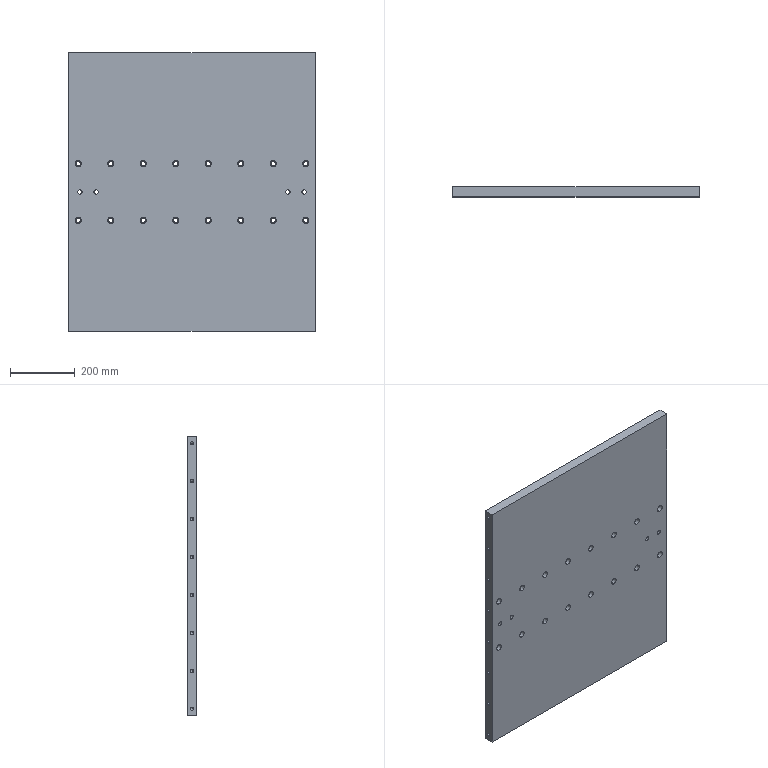Part | SolidWorks | features HoleWzd 4, Extrusion 1 | 1 solid | 170 faces | box 763 x 30 x 860 mm | volume 19515474 mm3 | cylinder 112 | cone 32 | plane 26 | commonest cylinder face diameters 13.5 x40 20 x40 10.2 x32